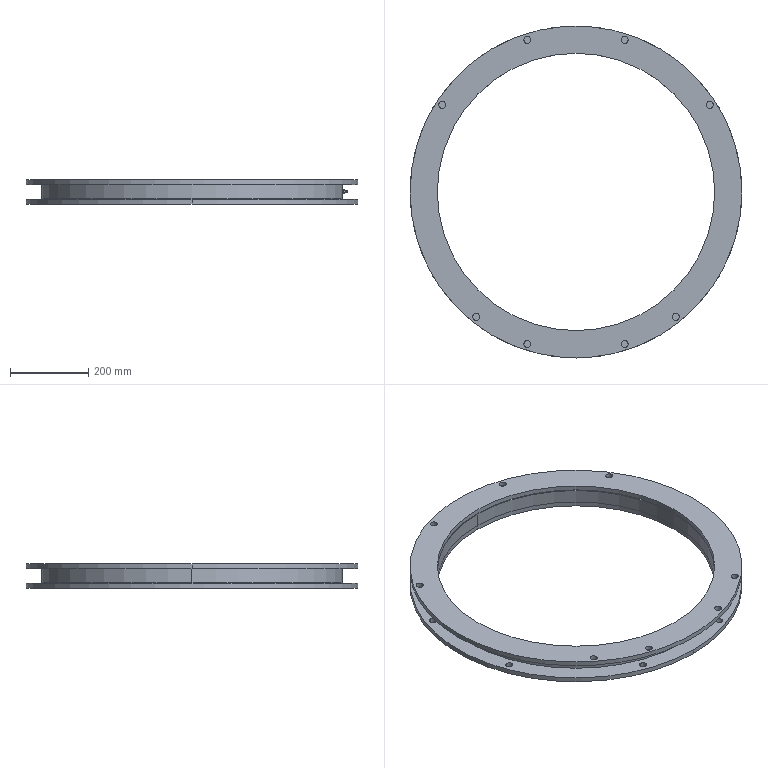Part | SolidWorks | features ReferencePattern 139, CompositeCurve 9, LocalCirPattern 1 | 145 solids | 391 faces | box 850 x 850 x 62 mm | volume 6412042 mm3 | sphere 284 | cylinder 60 | cone 20 | plane 19 | torus 8 | commonest cylinder face diameters 18 x32 740 x8 710 x6 850 x4 1.5 x2 3 x2